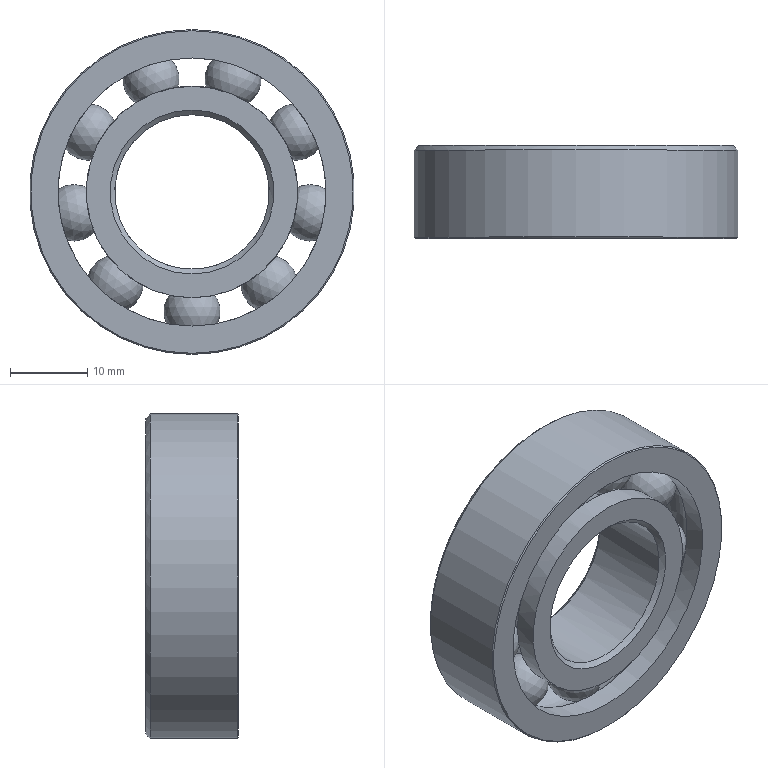Part | STEP file | 冲床-300配套压波_id1046_x_t | 1 solid | 41 faces | box 42 x 12 x 42 mm | volume 8800 mm3 | torus 18 | sphere 9 | cylinder 6 | plane 4 | cone 4 | commonest cylinder face diameters 27.334 x2 34.666 x2 20 x1 42 x1